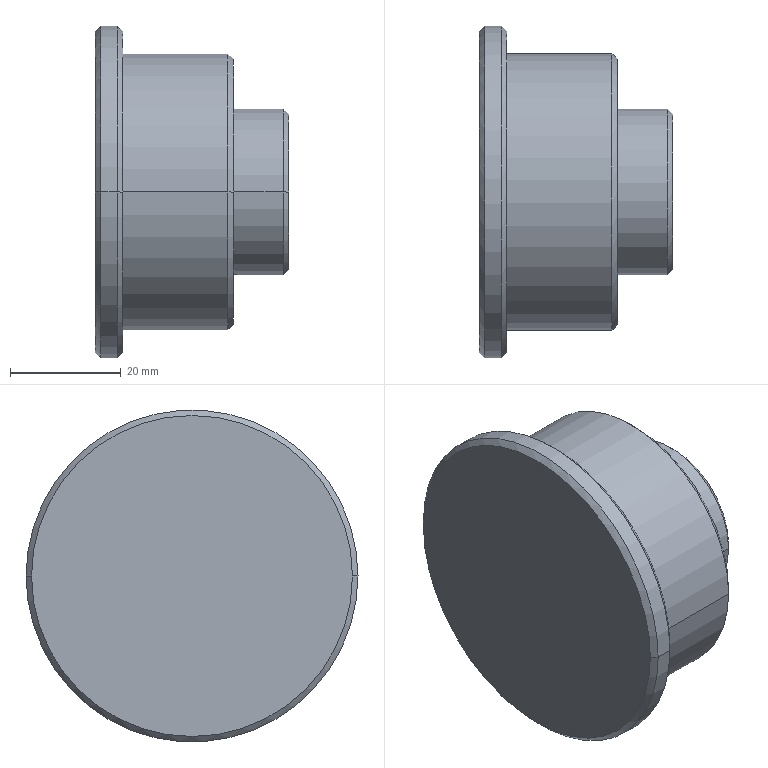Part | SolidWorks | features Chamfer 1, Revolution 1 | 1 solid | 18 faces | box 35 x 60 x 60 mm | volume 60166 mm3 | cone 8 | cylinder 6 | plane 4 | commonest cylinder face diameters 30 x2 50 x2 60 x2
STEP:
#1=CARTESIAN_POINT('',(30.,14.,0.));
#2=VERTEX_POINT('',#1);
#3=CARTESIAN_POINT('',(30.,-14.,0.));
#4=VERTEX_POINT('',#3);
#5=CARTESIAN_POINT('',(30.,0.,0.));
#6=DIRECTION('',(1.,0.,0.));
#7=DIRECTION('',(0.,-1.,0.));
#8=AXIS2_PLACEMENT_3D('',#5,#6,#7);
#9=CIRCLE('',#8,14.);
#10=EDGE_CURVE('',#2,#4,#9,.T.);
#11=ORIENTED_EDGE('',*,*,#10,.F.);
#12=CARTESIAN_POINT('',(29.,15.,0.));
#13=VERTEX_POINT('',#12);
#14=CARTESIAN_POINT('',(30.,14.,0.));
#15=DIRECTION('',(-0.7071,0.7071,0.));
#16=VECTOR('',#15,1000.);
#17=LINE('',#14,#16);
#18=EDGE_CURVE('',#2,#13,#17,.T.);
#19=ORIENTED_EDGE('',*,*,#18,.T.);
#20=CARTESIAN_POINT('',(29.,-15.,0.));
#21=VERTEX_POINT('',#20);
#22=CARTESIAN_POINT('',(29.,0.,0.));
#23=DIRECTION('',(-1.,0.,0.));
#24=DIRECTION('',(0.,-1.,0.));
#25=AXIS2_PLACEMENT_3D('',#22,#23,#24);
#26=CIRCLE('',#25,15.);
#27=EDGE_CURVE('',#21,#13,#26,.T.);
#28=ORIENTED_EDGE('',*,*,#27,.F.);
#29=CARTESIAN_POINT('',(30.,-14.,0.));
#30=DIRECTION('',(-0.7071,-0.7071,0.));
#31=VECTOR('',#30,1000.);
#32=LINE('',#29,#31);
#33=EDGE_CURVE('',#4,#21,#32,.T.);
#34=ORIENTED_EDGE('',*,*,#33,.F.);
#35=EDGE_LOOP('',(#11,#19,#28,#34));
#36=FACE_OUTER_BOUND('',#35,.T.);
#37=CARTESIAN_POINT('',(30.,0.,0.));
#38=DIRECTION('',(-1.,0.,0.));
#39=DIRECTION('',(0.,-1.,0.));
#40=AXIS2_PLACEMENT_3D('',#37,#38,#39);
#41=CONICAL_SURFACE('',#40,14.,0.7854);
#42=ADVANCED_FACE('',(#36),#41,.T.);
#43=CARTESIAN_POINT('',(20.,24.,0.));
#44=VERTEX_POINT('',#43);
#45=CARTESIAN_POINT('',(20.,-24.,0.));
#46=VERTEX_POINT('',#45);
#47=CARTESIAN_POINT('',(20.,0.,0.));
#48=DIRECTION('',(1.,0.,0.));
#49=DIRECTION('',(0.,-1.,0.));
#50=AXIS2_PLACEMENT_3D('',#47,#48,#49);
#51=CIRCLE('',#50,24.);
#52=EDGE_CURVE('',#44,#46,#51,.T.);
#53=ORIENTED_EDGE('',*,*,#52,.F.);
#54=CARTESIAN_POINT('',(19.,25.,0.));
#55=VERTEX_POINT('',#54);
#56=CARTESIAN_POINT('',(20.,24.,0.));
#57=DIRECTION('',(-0.7071,0.7071,0.));
#58=VECTOR('',#57,1000.);
#59=LINE('',#56,#58);
#60=EDGE_CURVE('',#44,#55,#59,.T.);
#61=ORIENTED_EDGE('',*,*,#60,.T.);
#62=CARTESIAN_POINT('',(19.,-25.,0.));
#63=VERTEX_POINT('',#62);
#64=CARTESIAN_POINT('',(19.,0.,0.));
#65=DIRECTION('',(-1.,0.,0.));
#66=DIRECTION('',(0.,-1.,0.));
#67=AXIS2_PLACEMENT_3D('',#64,#65,#66);
#68=CIRCLE('',#67,25.);
#69=EDGE_CURVE('',#63,#55,#68,.T.);
#70=ORIENTED_EDGE('',*,*,#69,.F.);
#71=CARTESIAN_POINT('',(20.,-24.,0.));
#72=DIRECTION('',(-0.7071,-0.7071,0.));
#73=VECTOR('',#72,1000.);
#74=LINE('',#71,#73);
#75=EDGE_CURVE('',#46,#63,#74,.T.);
#76=ORIENTED_EDGE('',*,*,#75,.F.);
#77=EDGE_LOOP('',(#53,#61,#70,#76));
#78=FACE_OUTER_BOUND('',#77,.T.);
#79=CARTESIAN_POINT('',(20.,0.,0.));
#80=DIRECTION('',(-1.,0.,0.));
#81=DIRECTION('',(0.,-1.,0.));
#82=AXIS2_PLACEMENT_3D('',#79,#80,#81);
#83=CONICAL_SURFACE('',#82,24.,0.7854);
#84=ADVANCED_FACE('',(#78),#83,.T.);
#85=CARTESIAN_POINT('',(0.,29.,0.));
#86=VERTEX_POINT('',#85);
#87=CARTESIAN_POINT('',(0.,-29.,0.));
#88=VERTEX_POINT('',#87);
#89=CARTESIAN_POINT('',(0.,0.,0.));
#90=DIRECTION('',(1.,0.,0.));
#91=DIRECTION('',(0.,-1.,0.));
#92=AXIS2_PLACEMENT_3D('',#89,#90,#91);
#93=CIRCLE('',#92,29.);
#94=EDGE_CURVE('',#86,#88,#93,.T.);
#95=ORIENTED_EDGE('',*,*,#94,.F.);
#96=CARTESIAN_POINT('',(-1.,30.,0.));
#97=VERTEX_POINT('',#96);
#98=CARTESIAN_POINT('',(0.,29.,0.));
#99=DIRECTION('',(-0.7071,0.7071,0.));
#100=VECTOR('',#99,1000.);
#101=LINE('',#98,#100);
#102=EDGE_CURVE('',#86,#97,#101,.T.);
#103=ORIENTED_EDGE('',*,*,#102,.T.);
#104=CARTESIAN_POINT('',(-1.,-30.,0.));
#105=VERTEX_POINT('',#104);
#106=CARTESIAN_POINT('',(-1.,0.,0.));
#107=DIRECTION('',(-1.,0.,0.));
#108=DIRECTION('',(0.,-1.,0.));
#109=AXIS2_PLACEMENT_3D('',#106,#107,#108);
#110=CIRCLE('',#109,30.);
#111=EDGE_CURVE('',#105,#97,#110,.T.);
#112=ORIENTED_EDGE('',*,*,#111,.F.);
#113=CARTESIAN_POINT('',(0.,-29.,0.));
#114=DIRECTION('',(-0.7071,-0.7071,0.));
#115=VECTOR('',#114,1000.);
#116=LINE('',#113,#115);
#117=EDGE_CURVE('',#88,#105,#116,.T.);
#118=ORIENTED_EDGE('',*,*,#117,.F.);
#119=EDGE_LOOP('',(#95,#103,#112,#118));
#120=FACE_OUTER_BOUND('',#119,.T.);
#121=CARTESIAN_POINT('',(0.,0.,0.));
#122=DIRECTION('',(-1.,0.,0.));
#123=DIRECTION('',(0.,-1.,0.));
#124=AXIS2_PLACEMENT_3D('',#121,#122,#123);
#125=CONICAL_SURFACE('',#124,29.,0.7854);
#126=ADVANCED_FACE('',(#120),#125,.T.);
#127=CARTESIAN_POINT('',(-5.,-29.,0.));
#128=VERTEX_POINT('',#127);
#129=CARTESIAN_POINT('',(-5.,29.,0.));
#130=VERTEX_POINT('',#129);
#131=CARTESIAN_POINT('',(-5.,0.,0.));
#132=DIRECTION('',(-1.,0.,0.));
#133=DIRECTION('',(0.,1.,0.));
#134=AXIS2_PLACEMENT_3D('',#131,#132,#133);
#135=CIRCLE('',#134,29.);
#136=EDGE_CURVE('',#128,#130,#135,.T.);
#137=ORIENTED_EDGE('',*,*,#136,.F.);
#138=CARTESIAN_POINT('',(-4.,-30.,0.));
#139=VERTEX_POINT('',#138);
#140=CARTESIAN_POINT('',(-4.,-30.,0.));
#141=DIRECTION('',(0.7071,-0.7071,0.));
#142=VECTOR('',#141,1000.);
#143=LINE('',#140,#142);
#144=EDGE_CURVE('',#128,#139,#143,.T.);
#145=ORIENTED_EDGE('',*,*,#144,.T.);
#146=CARTESIAN_POINT('',(-4.,30.,0.));
#147=VERTEX_POINT('',#146);
#148=CARTESIAN_POINT('',(-4.,0.,0.));
#149=DIRECTION('',(1.,0.,0.));
#150=DIRECTION('',(0.,1.,0.));
#151=AXIS2_PLACEMENT_3D('',#148,#149,#150);
#152=CIRCLE('',#151,30.);
#153=EDGE_CURVE('',#147,#139,#152,.T.);
#154=ORIENTED_EDGE('',*,*,#153,.F.);
#155=CARTESIAN_POINT('',(-4.,30.,0.));
#156=DIRECTION('',(0.7071,0.7071,0.));
#157=VECTOR('',#156,1000.);
#158=LINE('',#155,#157);
#159=EDGE_CURVE('',#130,#147,#158,.T.);
#160=ORIENTED_EDGE('',*,*,#159,.F.);
#161=EDGE_LOOP('',(#137,#145,#154,#160));
#162=FACE_OUTER_BOUND('',#161,.T.);
#163=CARTESIAN_POINT('',(-4.,0.,0.));
#164=DIRECTION('',(1.,0.,0.));
#165=DIRECTION('',(0.,1.,0.));
#166=AXIS2_PLACEMENT_3D('',#163,#164,#165);
#167=CONICAL_SURFACE('',#166,30.,0.7854);
#168=ADVANCED_FACE('',(#162),#167,.T.);
#169=CARTESIAN_POINT('',(20.,15.,0.));
#170=VERTEX_POINT('',#169);
#171=CARTESIAN_POINT('',(20.,-15.,0.));
#172=VERTEX_POINT('',#171);
#173=CARTESIAN_POINT('',(20.,0.,0.));
#174=DIRECTION('',(1.,0.,0.));
#175=DIRECTION('',(0.,1.,0.));
#176=AXIS2_PLACEMENT_3D('',#173,#174,#175);
#177=CIRCLE('',#176,15.);
#178=EDGE_CURVE('',#170,#172,#177,.T.);
#179=ORIENTED_EDGE('',*,*,#178,.T.);
#180=CARTESIAN_POINT('',(30.,-15.,0.));
#181=DIRECTION('',(1.,0.,0.));
#182=VECTOR('',#181,1000.);
#183=LINE('',#180,#182);
#184=EDGE_CURVE('',#172,#21,#183,.T.);
#185=ORIENTED_EDGE('',*,*,#184,.T.);
#186=ORIENTED_EDGE('',*,*,#27,.T.);
#187=CARTESIAN_POINT('',(30.,15.,0.));
#188=DIRECTION('',(1.,0.,0.));
#189=VECTOR('',#188,1000.);
#190=LINE('',#187,#189);
#191=EDGE_CURVE('',#170,#13,#190,.T.);
#192=ORIENTED_EDGE('',*,*,#191,.F.);
#193=EDGE_LOOP('',(#179,#185,#186,#192));
#194=FACE_OUTER_BOUND('',#193,.T.);
#195=CARTESIAN_POINT('',(30.,0.,0.));
#196=DIRECTION('',(1.,0.,0.));
#197=DIRECTION('',(0.,1.,0.));
#198=AXIS2_PLACEMENT_3D('',#195,#196,#197);
#199=CYLINDRICAL_SURFACE('',#198,15.);
#200=ADVANCED_FACE('',(#194),#199,.T.);
#201=CARTESIAN_POINT('',(0.,25.,0.));
#202=VERTEX_POINT('',#201);
#203=CARTESIAN_POINT('',(0.,-25.,0.));
#204=VERTEX_POINT('',#203);
#205=CARTESIAN_POINT('',(0.,0.,0.));
#206=DIRECTION('',(1.,0.,0.));
#207=DIRECTION('',(0.,1.,0.));
#208=AXIS2_PLACEMENT_3D('',#205,#206,#207);
#209=CIRCLE('',#208,25.);
#210=EDGE_CURVE('',#202,#204,#209,.T.);
#211=ORIENTED_EDGE('',*,*,#210,.T.);
#212=CARTESIAN_POINT('',(30.,-25.,0.));
#213=DIRECTION('',(1.,0.,0.));
#214=VECTOR('',#213,1000.);
#215=LINE('',#212,#214);
#216=EDGE_CURVE('',#204,#63,#215,.T.);
#217=ORIENTED_EDGE('',*,*,#216,.T.);
#218=ORIENTED_EDGE('',*,*,#69,.T.);
#219=CARTESIAN_POINT('',(30.,25.,0.));
#220=DIRECTION('',(1.,0.,0.));
#221=VECTOR('',#220,1000.);
#222=LINE('',#219,#221);
#223=EDGE_CURVE('',#202,#55,#222,.T.);
#224=ORIENTED_EDGE('',*,*,#223,.F.);
#225=EDGE_LOOP('',(#211,#217,#218,#224));
#226=FACE_OUTER_BOUND('',#225,.T.);
#227=CARTESIAN_POINT('',(30.,0.,0.));
#228=DIRECTION('',(1.,0.,0.));
#229=DIRECTION('',(0.,1.,0.));
#230=AXIS2_PLACEMENT_3D('',#227,#228,#229);
#231=CYLINDRICAL_SURFACE('',#230,25.);
#232=ADVANCED_FACE('',(#226),#231,.T.);
#233=ORIENTED_EDGE('',*,*,#153,.T.);
#234=CARTESIAN_POINT('',(30.,-30.,0.));
#235=DIRECTION('',(1.,0.,0.));
#236=VECTOR('',#235,1000.);
#237=LINE('',#234,#236);
#238=EDGE_CURVE('',#139,#105,#237,.T.);
#239=ORIENTED_EDGE('',*,*,#238,.T.);
#240=ORIENTED_EDGE('',*,*,#111,.T.);
#241=CARTESIAN_POINT('',(30.,30.,0.));
#242=DIRECTION('',(1.,0.,0.));
#243=VECTOR('',#242,1000.);
#244=LINE('',#241,#243);
#245=EDGE_CURVE('',#147,#97,#244,.T.);
#246=ORIENTED_EDGE('',*,*,#245,.F.);
#247=EDGE_LOOP('',(#233,#239,#240,#246));
#248=FACE_OUTER_BOUND('',#247,.T.);
#249=CARTESIAN_POINT('',(30.,0.,0.));
#250=DIRECTION('',(1.,0.,0.));
#251=DIRECTION('',(0.,1.,0.));
#252=AXIS2_PLACEMENT_3D('',#249,#250,#251);
#253=CYLINDRICAL_SURFACE('',#252,30.);
#254=ADVANCED_FACE('',(#248),#253,.T.);
#255=CARTESIAN_POINT('',(-5.,0.,0.));
#256=DIRECTION('',(-1.,0.,0.));
#257=DIRECTION('',(0.,1.,0.));
#258=AXIS2_PLACEMENT_3D('',#255,#256,#257);
#259=CIRCLE('',#258,29.);
#260=EDGE_CURVE('',#130,#128,#259,.T.);
#261=ORIENTED_EDGE('',*,*,#260,.T.);
#262=ORIENTED_EDGE('',*,*,#136,.T.);
#263=EDGE_LOOP('',(#261,#262));
#264=FACE_OUTER_BOUND('',#263,.T.);
#265=CARTESIAN_POINT('',(-5.,-30.,0.));
#266=DIRECTION('',(1.,0.,0.));
#267=DIRECTION('',(0.,1.,0.));
#268=AXIS2_PLACEMENT_3D('',#265,#266,#267);
#269=PLANE('',#268);
#270=ADVANCED_FACE('',(#264),#269,.F.);
#271=ORIENTED_EDGE('',*,*,#238,.F.);
#272=CARTESIAN_POINT('',(-4.,0.,0.));
#273=DIRECTION('',(1.,0.,0.));
#274=DIRECTION('',(0.,1.,0.));
#275=AXIS2_PLACEMENT_3D('',#272,#273,#274);
#276=CIRCLE('',#275,30.);
#277=EDGE_CURVE('',#139,#147,#276,.T.);
#278=ORIENTED_EDGE('',*,*,#277,.T.);
#279=ORIENTED_EDGE('',*,*,#245,.T.);
#280=CARTESIAN_POINT('',(-1.,0.,0.));
#281=DIRECTION('',(-1.,0.,0.));
#282=DIRECTION('',(0.,-1.,0.));
#283=AXIS2_PLACEMENT_3D('',#280,#281,#282);
#284=CIRCLE('',#283,30.);
#285=EDGE_CURVE('',#97,#105,#284,.T.);
#286=ORIENTED_EDGE('',*,*,#285,.T.);
#287=EDGE_LOOP('',(#271,#278,#279,#286));
#288=FACE_OUTER_BOUND('',#287,.T.);
#289=CARTESIAN_POINT('',(30.,0.,0.));
#290=DIRECTION('',(1.,0.,0.));
#291=DIRECTION('',(0.,1.,0.));
#292=AXIS2_PLACEMENT_3D('',#289,#290,#291);
#293=CYLINDRICAL_SURFACE('',#292,30.);
#294=ADVANCED_FACE('',(#288),#293,.T.);
#295=CARTESIAN_POINT('',(0.,0.,0.));
#296=DIRECTION('',(1.,0.,0.));
#297=DIRECTION('',(0.,-1.,0.));
#298=AXIS2_PLACEMENT_3D('',#295,#296,#297);
#299=CIRCLE('',#298,29.);
#300=EDGE_CURVE('',#88,#86,#299,.T.);
#301=ORIENTED_EDGE('',*,*,#300,.T.);
#302=ORIENTED_EDGE('',*,*,#94,.T.);
#303=EDGE_LOOP('',(#301,#302));
#304=FACE_OUTER_BOUND('',#303,.T.);
#305=ORIENTED_EDGE('',*,*,#210,.F.);
#306=CARTESIAN_POINT('',(0.,0.,0.));
#307=DIRECTION('',(1.,0.,0.));
#308=DIRECTION('',(0.,1.,0.));
#309=AXIS2_PLACEMENT_3D('',#306,#307,#308);
#310=CIRCLE('',#309,25.);
#311=EDGE_CURVE('',#204,#202,#310,.T.);
#312=ORIENTED_EDGE('',*,*,#311,.F.);
#313=EDGE_LOOP('',(#305,#312));
#314=FACE_BOUND('',#313,.T.);
#315=CARTESIAN_POINT('',(0.,-25.,0.));
#316=DIRECTION('',(-1.,0.,0.));
#317=DIRECTION('',(0.,-1.,0.));
#318=AXIS2_PLACEMENT_3D('',#315,#316,#317);
#319=PLANE('',#318);
#320=ADVANCED_FACE('',(#304,#314),#319,.F.);
#321=ORIENTED_EDGE('',*,*,#216,.F.);
#322=ORIENTED_EDGE('',*,*,#311,.T.);
#323=ORIENTED_EDGE('',*,*,#223,.T.);
#324=CARTESIAN_POINT('',(19.,0.,0.));
#325=DIRECTION('',(-1.,0.,0.));
#326=DIRECTION('',(0.,-1.,0.));
#327=AXIS2_PLACEMENT_3D('',#324,#325,#326);
#328=CIRCLE('',#327,25.);
#329=EDGE_CURVE('',#55,#63,#328,.T.);
#330=ORIENTED_EDGE('',*,*,#329,.T.);
#331=EDGE_LOOP('',(#321,#322,#323,#330));
#332=FACE_OUTER_BOUND('',#331,.T.);
#333=CARTESIAN_POINT('',(30.,0.,0.));
#334=DIRECTION('',(1.,0.,0.));
#335=DIRECTION('',(0.,1.,0.));
#336=AXIS2_PLACEMENT_3D('',#333,#334,#335);
#337=CYLINDRICAL_SURFACE('',#336,25.);
#338=ADVANCED_FACE('',(#332),#337,.T.);
#339=CARTESIAN_POINT('',(20.,0.,0.));
#340=DIRECTION('',(1.,0.,0.));
#341=DIRECTION('',(0.,-1.,0.));
#342=AXIS2_PLACEMENT_3D('',#339,#340,#341);
#343=CIRCLE('',#342,24.);
#344=EDGE_CURVE('',#46,#44,#343,.T.);
#345=ORIENTED_EDGE('',*,*,#344,.T.);
#346=ORIENTED_EDGE('',*,*,#52,.T.);
#347=EDGE_LOOP('',(#345,#346));
#348=FACE_OUTER_BOUND('',#347,.T.);
#349=ORIENTED_EDGE('',*,*,#178,.F.);
#350=CARTESIAN_POINT('',(20.,0.,0.));
#351=DIRECTION('',(1.,0.,0.));
#352=DIRECTION('',(0.,1.,0.));
#353=AXIS2_PLACEMENT_3D('',#350,#351,#352);
#354=CIRCLE('',#353,15.);
#355=EDGE_CURVE('',#172,#170,#354,.T.);
#356=ORIENTED_EDGE('',*,*,#355,.F.);
#357=EDGE_LOOP('',(#349,#356));
#358=FACE_BOUND('',#357,.T.);
#359=CARTESIAN_POINT('',(20.,-15.,0.));
#360=DIRECTION('',(-1.,0.,0.));
#361=DIRECTION('',(0.,-1.,0.));
#362=AXIS2_PLACEMENT_3D('',#359,#360,#361);
#363=PLANE('',#362);
#364=ADVANCED_FACE('',(#348,#358),#363,.F.);
#365=ORIENTED_EDGE('',*,*,#184,.F.);
#366=ORIENTED_EDGE('',*,*,#355,.T.);
#367=ORIENTED_EDGE('',*,*,#191,.T.);
#368=CARTESIAN_POINT('',(29.,0.,0.));
#369=DIRECTION('',(-1.,0.,0.));
#370=DIRECTION('',(0.,-1.,0.));
#371=AXIS2_PLACEMENT_3D('',#368,#369,#370);
#372=CIRCLE('',#371,15.);
#373=EDGE_CURVE('',#13,#21,#372,.T.);
#374=ORIENTED_EDGE('',*,*,#373,.T.);
#375=EDGE_LOOP('',(#365,#366,#367,#374));
#376=FACE_OUTER_BOUND('',#375,.T.);
#377=CARTESIAN_POINT('',(30.,0.,0.));
#378=DIRECTION('',(1.,0.,0.));
#379=DIRECTION('',(0.,1.,0.));
#380=AXIS2_PLACEMENT_3D('',#377,#378,#379);
#381=CYLINDRICAL_SURFACE('',#380,15.);
#382=ADVANCED_FACE('',(#376),#381,.T.);
#383=CARTESIAN_POINT('',(30.,0.,0.));
#384=DIRECTION('',(1.,0.,0.));
#385=DIRECTION('',(0.,-1.,0.));
#386=AXIS2_PLACEMENT_3D('',#383,#384,#385);
#387=CIRCLE('',#386,14.);
#388=EDGE_CURVE('',#4,#2,#387,.T.);
#389=ORIENTED_EDGE('',*,*,#388,.T.);
#390=ORIENTED_EDGE('',*,*,#10,.T.);
#391=EDGE_LOOP('',(#389,#390));
#392=FACE_OUTER_BOUND('',#391,.T.);
#393=CARTESIAN_POINT('',(30.,-15.,0.));
#394=DIRECTION('',(-1.,0.,0.));
#395=DIRECTION('',(0.,-1.,0.));
#396=AXIS2_PLACEMENT_3D('',#393,#394,#395);
#397=PLANE('',#396);
#398=ADVANCED_FACE('',(#392),#397,.F.);
#399=ORIENTED_EDGE('',*,*,#144,.F.);
#400=ORIENTED_EDGE('',*,*,#260,.F.);
#401=ORIENTED_EDGE('',*,*,#159,.T.);
#402=ORIENTED_EDGE('',*,*,#277,.F.);
#403=EDGE_LOOP('',(#399,#400,#401,#402));
#404=FACE_OUTER_BOUND('',#403,.T.);
#405=CARTESIAN_POINT('',(-4.,0.,0.));
#406=DIRECTION('',(1.,0.,0.));
#407=DIRECTION('',(0.,1.,0.));
#408=AXIS2_PLACEMENT_3D('',#405,#406,#407);
#409=CONICAL_SURFACE('',#408,30.,0.7854);
#410=ADVANCED_FACE('',(#404),#409,.T.);
#411=ORIENTED_EDGE('',*,*,#102,.F.);
#412=ORIENTED_EDGE('',*,*,#300,.F.);
#413=ORIENTED_EDGE('',*,*,#117,.T.);
#414=ORIENTED_EDGE('',*,*,#285,.F.);
#415=EDGE_LOOP('',(#411,#412,#413,#414));
#416=FACE_OUTER_BOUND('',#415,.T.);
#417=CARTESIAN_POINT('',(0.,0.,0.));
#418=DIRECTION('',(-1.,0.,0.));
#419=DIRECTION('',(0.,-1.,0.));
#420=AXIS2_PLACEMENT_3D('',#417,#418,#419);
#421=CONICAL_SURFACE('',#420,29.,0.7854);
#422=ADVANCED_FACE('',(#416),#421,.T.);
#423=ORIENTED_EDGE('',*,*,#60,.F.);
#424=ORIENTED_EDGE('',*,*,#344,.F.);
#425=ORIENTED_EDGE('',*,*,#75,.T.);
#426=ORIENTED_EDGE('',*,*,#329,.F.);
#427=EDGE_LOOP('',(#423,#424,#425,#426));
#428=FACE_OUTER_BOUND('',#427,.T.);
#429=CARTESIAN_POINT('',(20.,0.,0.));
#430=DIRECTION('',(-1.,0.,0.));
#431=DIRECTION('',(0.,-1.,0.));
#432=AXIS2_PLACEMENT_3D('',#429,#430,#431);
#433=CONICAL_SURFACE('',#432,24.,0.7854);
#434=ADVANCED_FACE('',(#428),#433,.T.);
#435=ORIENTED_EDGE('',*,*,#18,.F.);
#436=ORIENTED_EDGE('',*,*,#388,.F.);
#437=ORIENTED_EDGE('',*,*,#33,.T.);
#438=ORIENTED_EDGE('',*,*,#373,.F.);
#439=EDGE_LOOP('',(#435,#436,#437,#438));
#440=FACE_OUTER_BOUND('',#439,.T.);
#441=CARTESIAN_POINT('',(30.,0.,0.));
#442=DIRECTION('',(-1.,0.,0.));
#443=DIRECTION('',(0.,-1.,0.));
#444=AXIS2_PLACEMENT_3D('',#441,#442,#443);
#445=CONICAL_SURFACE('',#444,14.,0.7854);
#446=ADVANCED_FACE('',(#440),#445,.T.);
#447=CLOSED_SHELL('',(#42,#84,#126,#168,#200,#232,#254,#270,#294,#320,#338,#364,#382,#398,#410,#422,#434,#446));
#448=MANIFOLD_SOLID_BREP('',#447);
#449=CARTESIAN_POINT('',(0.,0.,0.));
#450=DIRECTION('',(0.,0.,1.));
#451=DIRECTION('',(1.,0.,0.));
#452=AXIS2_PLACEMENT_3D('',#449,#450,#451);
#453=(LENGTH_UNIT()NAMED_UNIT(*)SI_UNIT(.MILLI.,.METRE.));
#454=UNCERTAINTY_MEASURE_WITH_UNIT(LENGTH_MEASURE(0.00001),#453,'','');
#455=(NAMED_UNIT(*)PLANE_ANGLE_UNIT()SI_UNIT($,.RADIAN.));
#456=(NAMED_UNIT(*)SI_UNIT($,.STERADIAN.)SOLID_ANGLE_UNIT());
#457=(GEOMETRIC_REPRESENTATION_CONTEXT(3)GLOBAL_UNCERTAINTY_ASSIGNED_CONTEXT((#454))GLOBAL_UNIT_ASSIGNED_CONTEXT((#453,#455,#456))REPRESENTATION_CONTEXT('',''));
#458=ADVANCED_BREP_SHAPE_REPRESENTATION('',(#448,#452),#457);